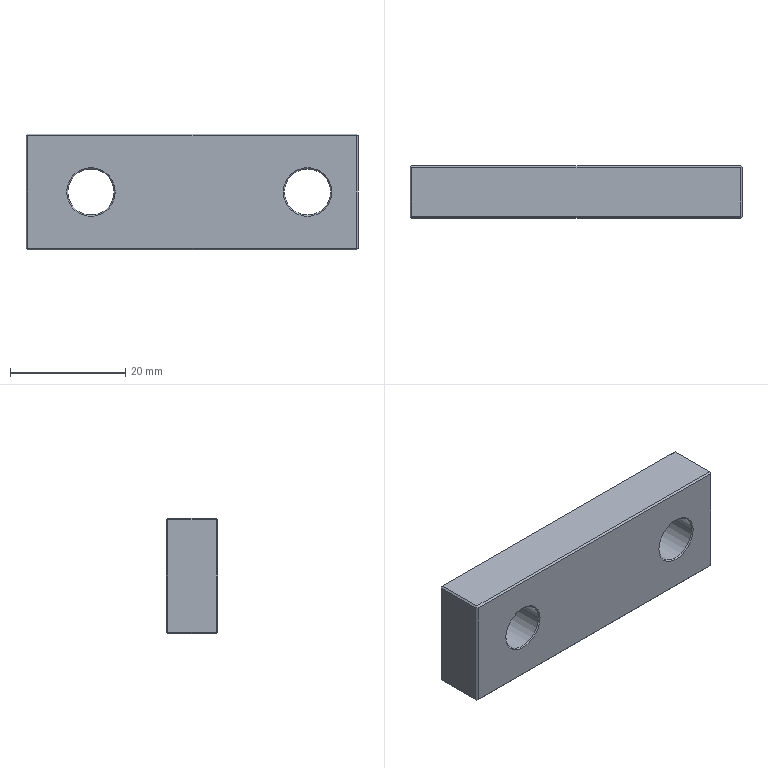Part | 1 solid | 26 faces | box 57.5 x 9 x 20 mm | volume 9429 mm3 | plane 18 | cylinder 4 | cone 4 | commonest cylinder face diameters 8 x4
STEP:
#1=CARTESIAN_POINT('',(2209.7,120.2,40.));
#2=VERTEX_POINT('',#1);
#3=CARTESIAN_POINT('',(2209.7,111.8,40.));
#4=VERTEX_POINT('',#3);
#5=CARTESIAN_POINT('',(2209.7,116.,40.));
#6=DIRECTION('',(0.,-1.,0.));
#7=VECTOR('',#6,1000.);
#8=LINE('',#5,#7);
#9=EDGE_CURVE('',#2,#4,#8,.T.);
#10=ORIENTED_EDGE('',*,*,#9,.T.);
#11=CARTESIAN_POINT('',(2152.8,111.8,40.));
#12=VERTEX_POINT('',#11);
#13=CARTESIAN_POINT('',(2184.262,111.8,40.));
#14=DIRECTION('',(1.,0.,0.));
#15=VECTOR('',#14,1000.);
#16=LINE('',#13,#15);
#17=EDGE_CURVE('',#12,#4,#16,.T.);
#18=ORIENTED_EDGE('',*,*,#17,.F.);
#19=CARTESIAN_POINT('',(2152.8,120.2,40.));
#20=VERTEX_POINT('',#19);
#21=CARTESIAN_POINT('',(2152.8,110.5,40.));
#22=DIRECTION('',(0.,-1.,0.));
#23=VECTOR('',#22,1000.);
#24=LINE('',#21,#23);
#25=EDGE_CURVE('',#20,#12,#24,.T.);
#26=ORIENTED_EDGE('',*,*,#25,.F.);
#27=CARTESIAN_POINT('',(2184.262,120.2,40.));
#28=DIRECTION('',(-1.,0.,0.));
#29=VECTOR('',#28,1000.);
#30=LINE('',#27,#29);
#31=EDGE_CURVE('',#2,#20,#30,.T.);
#32=ORIENTED_EDGE('',*,*,#31,.F.);
#33=EDGE_LOOP('',(#10,#18,#26,#32));
#34=FACE_BOUND('',#33,.T.);
#35=CARTESIAN_POINT('',(2131.5,110.5,40.));
#36=DIRECTION('',(0.,0.,-1.));
#37=DIRECTION('',(0.,-1.,0.));
#38=AXIS2_PLACEMENT_3D('',#35,#36,#37);
#39=PLANE('',#38);
#40=ADVANCED_FACE('',(#34),#39,.T.);
#41=CARTESIAN_POINT('',(2152.5,111.8,59.7));
#42=VERTEX_POINT('',#41);
#43=CARTESIAN_POINT('',(2152.5,120.2,59.7));
#44=VERTEX_POINT('',#43);
#45=CARTESIAN_POINT('',(2152.5,110.5,59.7));
#46=DIRECTION('',(0.,1.,0.));
#47=VECTOR('',#46,1000.);
#48=LINE('',#45,#47);
#49=EDGE_CURVE('',#42,#44,#48,.T.);
#50=ORIENTED_EDGE('',*,*,#49,.T.);
#51=CARTESIAN_POINT('',(2152.5,120.2,40.3));
#52=VERTEX_POINT('',#51);
#53=CARTESIAN_POINT('',(2152.5,120.2,50.));
#54=DIRECTION('',(0.,0.,1.));
#55=VECTOR('',#54,1000.);
#56=LINE('',#53,#55);
#57=EDGE_CURVE('',#52,#44,#56,.T.);
#58=ORIENTED_EDGE('',*,*,#57,.F.);
#59=CARTESIAN_POINT('',(2152.5,111.8,40.3));
#60=VERTEX_POINT('',#59);
#61=CARTESIAN_POINT('',(2152.5,110.5,40.3));
#62=DIRECTION('',(0.,-1.,0.));
#63=VECTOR('',#62,1000.);
#64=LINE('',#61,#63);
#65=EDGE_CURVE('',#52,#60,#64,.T.);
#66=ORIENTED_EDGE('',*,*,#65,.T.);
#67=CARTESIAN_POINT('',(2152.5,111.8,50.));
#68=DIRECTION('',(0.,0.,-1.));
#69=VECTOR('',#68,1000.);
#70=LINE('',#67,#69);
#71=EDGE_CURVE('',#42,#60,#70,.T.);
#72=ORIENTED_EDGE('',*,*,#71,.F.);
#73=EDGE_LOOP('',(#50,#58,#66,#72));
#74=FACE_BOUND('',#73,.T.);
#75=CARTESIAN_POINT('',(2152.5,110.5,62.5));
#76=DIRECTION('',(-1.,0.,0.));
#77=DIRECTION('',(0.,0.,1.));
#78=AXIS2_PLACEMENT_3D('',#75,#76,#77);
#79=PLANE('',#78);
#80=ADVANCED_FACE('',(#74),#79,.T.);
#81=CARTESIAN_POINT('',(2209.7,111.8,60.));
#82=VERTEX_POINT('',#81);
#83=CARTESIAN_POINT('',(2209.7,120.2,60.));
#84=VERTEX_POINT('',#83);
#85=CARTESIAN_POINT('',(2209.7,116.,60.));
#86=DIRECTION('',(0.,1.,0.));
#87=VECTOR('',#86,1000.);
#88=LINE('',#85,#87);
#89=EDGE_CURVE('',#82,#84,#88,.T.);
#90=ORIENTED_EDGE('',*,*,#89,.T.);
#91=CARTESIAN_POINT('',(2152.8,120.2,60.));
#92=VERTEX_POINT('',#91);
#93=CARTESIAN_POINT('',(2184.262,120.2,60.));
#94=DIRECTION('',(1.,0.,0.));
#95=VECTOR('',#94,1000.);
#96=LINE('',#93,#95);
#97=EDGE_CURVE('',#92,#84,#96,.T.);
#98=ORIENTED_EDGE('',*,*,#97,.F.);
#99=CARTESIAN_POINT('',(2152.8,111.8,60.));
#100=VERTEX_POINT('',#99);
#101=CARTESIAN_POINT('',(2152.8,110.5,60.));
#102=DIRECTION('',(0.,1.,0.));
#103=VECTOR('',#102,1000.);
#104=LINE('',#101,#103);
#105=EDGE_CURVE('',#100,#92,#104,.T.);
#106=ORIENTED_EDGE('',*,*,#105,.F.);
#107=CARTESIAN_POINT('',(2184.262,111.8,60.));
#108=DIRECTION('',(-1.,0.,0.));
#109=VECTOR('',#108,1000.);
#110=LINE('',#107,#109);
#111=EDGE_CURVE('',#82,#100,#110,.T.);
#112=ORIENTED_EDGE('',*,*,#111,.F.);
#113=EDGE_LOOP('',(#90,#98,#106,#112));
#114=FACE_BOUND('',#113,.T.);
#115=CARTESIAN_POINT('',(2233.5,110.5,60.));
#116=DIRECTION('',(0.,0.,1.));
#117=DIRECTION('',(1.,0.,0.));
#118=AXIS2_PLACEMENT_3D('',#115,#116,#117);
#119=PLANE('',#118);
#120=ADVANCED_FACE('',(#114),#119,.T.);
#121=CARTESIAN_POINT('',(2210.,111.8,59.7));
#122=VERTEX_POINT('',#121);
#123=CARTESIAN_POINT('',(2210.,120.2,59.7));
#124=VERTEX_POINT('',#123);
#125=CARTESIAN_POINT('',(2210.,116.,59.7));
#126=DIRECTION('',(0.,1.,0.));
#127=VECTOR('',#126,1000.);
#128=LINE('',#125,#127);
#129=EDGE_CURVE('',#122,#124,#128,.T.);
#130=ORIENTED_EDGE('',*,*,#129,.F.);
#131=CARTESIAN_POINT('',(2210.,111.8,40.3));
#132=VERTEX_POINT('',#131);
#133=CARTESIAN_POINT('',(2210.,111.8,50.));
#134=DIRECTION('',(0.,0.,-1.));
#135=VECTOR('',#134,1000.);
#136=LINE('',#133,#135);
#137=EDGE_CURVE('',#122,#132,#136,.T.);
#138=ORIENTED_EDGE('',*,*,#137,.T.);
#139=CARTESIAN_POINT('',(2210.,120.2,40.3));
#140=VERTEX_POINT('',#139);
#141=CARTESIAN_POINT('',(2210.,116.,40.3));
#142=DIRECTION('',(0.,-1.,0.));
#143=VECTOR('',#142,1000.);
#144=LINE('',#141,#143);
#145=EDGE_CURVE('',#140,#132,#144,.T.);
#146=ORIENTED_EDGE('',*,*,#145,.F.);
#147=CARTESIAN_POINT('',(2210.,120.2,50.));
#148=DIRECTION('',(0.,0.,-1.));
#149=VECTOR('',#148,1000.);
#150=LINE('',#147,#149);
#151=EDGE_CURVE('',#124,#140,#150,.T.);
#152=ORIENTED_EDGE('',*,*,#151,.F.);
#153=EDGE_LOOP('',(#130,#138,#146,#152));
#154=FACE_BOUND('',#153,.T.);
#155=CARTESIAN_POINT('',(2210.,110.5,-72.5));
#156=DIRECTION('',(1.,0.,0.));
#157=DIRECTION('',(0.,1.,0.));
#158=AXIS2_PLACEMENT_3D('',#155,#156,#157);
#159=PLANE('',#158);
#160=ADVANCED_FACE('',(#154),#159,.T.);
#161=CARTESIAN_POINT('',(2197.25,111.7,50.));
#162=VERTEX_POINT('',#161);
#163=CARTESIAN_POINT('',(2205.25,111.7,50.));
#164=VERTEX_POINT('',#163);
#165=CARTESIAN_POINT('',(2201.25,111.7,50.));
#166=DIRECTION('',(0.,-1.,0.));
#167=DIRECTION('',(1.,0.,0.));
#168=AXIS2_PLACEMENT_3D('',#165,#166,#167);
#169=CIRCLE('',#168,4.);
#170=EDGE_CURVE('',#162,#164,#169,.T.);
#171=ORIENTED_EDGE('',*,*,#170,.T.);
#172=CARTESIAN_POINT('',(2205.25,120.5,50.));
#173=VERTEX_POINT('',#172);
#174=CARTESIAN_POINT('',(2205.25,105.5,50.));
#175=DIRECTION('',(0.,-1.,0.));
#176=VECTOR('',#175,1000.);
#177=LINE('',#174,#176);
#178=EDGE_CURVE('',#173,#164,#177,.T.);
#179=ORIENTED_EDGE('',*,*,#178,.F.);
#180=CARTESIAN_POINT('',(2197.25,120.5,50.));
#181=VERTEX_POINT('',#180);
#182=CARTESIAN_POINT('',(2201.25,120.5,50.));
#183=DIRECTION('',(0.,-1.,0.));
#184=DIRECTION('',(1.,0.,0.));
#185=AXIS2_PLACEMENT_3D('',#182,#183,#184);
#186=CIRCLE('',#185,4.);
#187=EDGE_CURVE('',#181,#173,#186,.T.);
#188=ORIENTED_EDGE('',*,*,#187,.F.);
#189=CARTESIAN_POINT('',(2197.25,105.5,50.));
#190=DIRECTION('',(0.,-1.,0.));
#191=VECTOR('',#190,1000.);
#192=LINE('',#189,#191);
#193=EDGE_CURVE('',#181,#162,#192,.T.);
#194=ORIENTED_EDGE('',*,*,#193,.T.);
#195=EDGE_LOOP('',(#171,#179,#188,#194));
#196=FACE_BOUND('',#195,.T.);
#197=CARTESIAN_POINT('',(2201.25,105.5,50.));
#198=DIRECTION('',(0.,-1.,0.));
#199=DIRECTION('',(1.,0.,0.));
#200=AXIS2_PLACEMENT_3D('',#197,#198,#199);
#201=CYLINDRICAL_SURFACE('',#200,4.);
#202=ADVANCED_FACE('',(#196),#201,.F.);
#203=ORIENTED_EDGE('',*,*,#89,.F.);
#204=CARTESIAN_POINT('',(2209.85,111.65,59.85));
#205=VERTEX_POINT('',#204);
#206=CARTESIAN_POINT('',(2211.,110.5,58.7));
#207=DIRECTION('',(0.5774,-0.5774,-0.5774));
#208=VECTOR('',#207,1000.);
#209=LINE('',#206,#208);
#210=EDGE_CURVE('',#82,#205,#209,.T.);
#211=ORIENTED_EDGE('',*,*,#210,.T.);
#212=CARTESIAN_POINT('',(2302.588,204.388,-32.888));
#213=DIRECTION('',(-0.5774,-0.5774,0.5774));
#214=VECTOR('',#213,1000.);
#215=LINE('',#212,#214);
#216=EDGE_CURVE('',#122,#205,#215,.T.);
#217=ORIENTED_EDGE('',*,*,#216,.F.);
#218=ORIENTED_EDGE('',*,*,#129,.T.);
#219=CARTESIAN_POINT('',(2209.85,120.35,59.85));
#220=VERTEX_POINT('',#219);
#221=CARTESIAN_POINT('',(2302.588,27.612,-32.888));
#222=DIRECTION('',(0.5774,-0.5774,-0.5774));
#223=VECTOR('',#222,1000.);
#224=LINE('',#221,#223);
#225=EDGE_CURVE('',#220,#124,#224,.T.);
#226=ORIENTED_EDGE('',*,*,#225,.F.);
#227=CARTESIAN_POINT('',(2200.,110.5,69.7));
#228=DIRECTION('',(-0.5774,-0.5774,0.5774));
#229=VECTOR('',#228,1000.);
#230=LINE('',#227,#229);
#231=EDGE_CURVE('',#220,#84,#230,.T.);
#232=ORIENTED_EDGE('',*,*,#231,.T.);
#233=EDGE_LOOP('',(#203,#211,#217,#218,#226,#232));
#234=FACE_BOUND('',#233,.T.);
#235=CARTESIAN_POINT('',(2209.85,116.,59.85));
#236=DIRECTION('',(0.7071,0.,0.7071));
#237=DIRECTION('',(0.,-1.,0.));
#238=AXIS2_PLACEMENT_3D('',#235,#236,#237);
#239=PLANE('',#238);
#240=ADVANCED_FACE('',(#234),#239,.T.);
#241=ORIENTED_EDGE('',*,*,#25,.T.);
#242=CARTESIAN_POINT('',(2152.65,111.65,40.15));
#243=VERTEX_POINT('',#242);
#244=CARTESIAN_POINT('',(2184.262,143.262,8.538));
#245=DIRECTION('',(-0.5774,-0.5774,0.5774));
#246=VECTOR('',#245,1000.);
#247=LINE('',#244,#246);
#248=EDGE_CURVE('',#12,#243,#247,.T.);
#249=ORIENTED_EDGE('',*,*,#248,.T.);
#250=CARTESIAN_POINT('',(2184.262,80.038,8.538));
#251=DIRECTION('',(-0.5774,0.5774,0.5774));
#252=VECTOR('',#251,1000.);
#253=LINE('',#250,#252);
#254=EDGE_CURVE('',#243,#60,#253,.T.);
#255=ORIENTED_EDGE('',*,*,#254,.T.);
#256=ORIENTED_EDGE('',*,*,#65,.F.);
#257=CARTESIAN_POINT('',(2152.65,120.35,40.15));
#258=VERTEX_POINT('',#257);
#259=CARTESIAN_POINT('',(2184.262,151.962,8.538));
#260=DIRECTION('',(-0.5774,-0.5774,0.5774));
#261=VECTOR('',#260,1000.);
#262=LINE('',#259,#261);
#263=EDGE_CURVE('',#258,#52,#262,.T.);
#264=ORIENTED_EDGE('',*,*,#263,.F.);
#265=CARTESIAN_POINT('',(2162.5,110.5,30.3));
#266=DIRECTION('',(-0.5774,0.5774,0.5774));
#267=VECTOR('',#266,1000.);
#268=LINE('',#265,#267);
#269=EDGE_CURVE('',#20,#258,#268,.T.);
#270=ORIENTED_EDGE('',*,*,#269,.F.);
#271=EDGE_LOOP('',(#241,#249,#255,#256,#264,#270));
#272=FACE_BOUND('',#271,.T.);
#273=CARTESIAN_POINT('',(2152.65,114.5,40.15));
#274=DIRECTION('',(0.7071,0.,0.7071));
#275=DIRECTION('',(0.,-1.,0.));
#276=AXIS2_PLACEMENT_3D('',#273,#274,#275);
#277=PLANE('',#276);
#278=ADVANCED_FACE('',(#272),#277,.F.);
#279=ORIENTED_EDGE('',*,*,#49,.F.);
#280=CARTESIAN_POINT('',(2152.65,111.65,59.85));
#281=VERTEX_POINT('',#280);
#282=CARTESIAN_POINT('',(2184.262,80.038,91.462));
#283=DIRECTION('',(-0.5774,0.5774,-0.5774));
#284=VECTOR('',#283,1000.);
#285=LINE('',#282,#284);
#286=EDGE_CURVE('',#281,#42,#285,.T.);
#287=ORIENTED_EDGE('',*,*,#286,.F.);
#288=CARTESIAN_POINT('',(2151.5,110.5,58.7));
#289=DIRECTION('',(-0.5774,-0.5774,-0.5774));
#290=VECTOR('',#289,1000.);
#291=LINE('',#288,#290);
#292=EDGE_CURVE('',#100,#281,#291,.T.);
#293=ORIENTED_EDGE('',*,*,#292,.F.);
#294=ORIENTED_EDGE('',*,*,#105,.T.);
#295=CARTESIAN_POINT('',(2152.65,120.35,59.85));
#296=VERTEX_POINT('',#295);
#297=CARTESIAN_POINT('',(2162.5,110.5,69.7));
#298=DIRECTION('',(-0.5774,0.5774,-0.5774));
#299=VECTOR('',#298,1000.);
#300=LINE('',#297,#299);
#301=EDGE_CURVE('',#92,#296,#300,.T.);
#302=ORIENTED_EDGE('',*,*,#301,.T.);
#303=CARTESIAN_POINT('',(2142.8,110.5,50.));
#304=DIRECTION('',(0.5774,0.5774,0.5774));
#305=VECTOR('',#304,1000.);
#306=LINE('',#303,#305);
#307=EDGE_CURVE('',#44,#296,#306,.T.);
#308=ORIENTED_EDGE('',*,*,#307,.F.);
#309=EDGE_LOOP('',(#279,#287,#293,#294,#302,#308));
#310=FACE_BOUND('',#309,.T.);
#311=CARTESIAN_POINT('',(2152.65,114.5,59.85));
#312=DIRECTION('',(-0.7071,0.,0.7071));
#313=DIRECTION('',(0.,1.,0.));
#314=AXIS2_PLACEMENT_3D('',#311,#312,#313);
#315=PLANE('',#314);
#316=ADVANCED_FACE('',(#310),#315,.T.);
#317=ORIENTED_EDGE('',*,*,#9,.F.);
#318=CARTESIAN_POINT('',(2209.85,120.35,40.15));
#319=VERTEX_POINT('',#318);
#320=CARTESIAN_POINT('',(2200.,110.5,30.3));
#321=DIRECTION('',(0.5774,0.5774,0.5774));
#322=VECTOR('',#321,1000.);
#323=LINE('',#320,#322);
#324=EDGE_CURVE('',#2,#319,#323,.T.);
#325=ORIENTED_EDGE('',*,*,#324,.T.);
#326=CARTESIAN_POINT('',(2219.7,110.5,50.));
#327=DIRECTION('',(-0.5774,0.5774,-0.5774));
#328=VECTOR('',#327,1000.);
#329=LINE('',#326,#328);
#330=EDGE_CURVE('',#140,#319,#329,.T.);
#331=ORIENTED_EDGE('',*,*,#330,.F.);
#332=ORIENTED_EDGE('',*,*,#145,.T.);
#333=CARTESIAN_POINT('',(2209.85,111.65,40.15));
#334=VERTEX_POINT('',#333);
#335=CARTESIAN_POINT('',(2184.262,86.062,14.562));
#336=DIRECTION('',(-0.5774,-0.5774,-0.5774));
#337=VECTOR('',#336,1000.);
#338=LINE('',#335,#337);
#339=EDGE_CURVE('',#132,#334,#338,.T.);
#340=ORIENTED_EDGE('',*,*,#339,.T.);
#341=CARTESIAN_POINT('',(2211.,110.5,41.3));
#342=DIRECTION('',(-0.5774,0.5774,-0.5774));
#343=VECTOR('',#342,1000.);
#344=LINE('',#341,#343);
#345=EDGE_CURVE('',#334,#4,#344,.T.);
#346=ORIENTED_EDGE('',*,*,#345,.T.);
#347=EDGE_LOOP('',(#317,#325,#331,#332,#340,#346));
#348=FACE_BOUND('',#347,.T.);
#349=CARTESIAN_POINT('',(2209.85,116.,40.15));
#350=DIRECTION('',(0.7071,0.,-0.7071));
#351=DIRECTION('',(0.,-1.,0.));
#352=AXIS2_PLACEMENT_3D('',#349,#350,#351);
#353=PLANE('',#352);
#354=ADVANCED_FACE('',(#348),#353,.T.);
#355=ORIENTED_EDGE('',*,*,#170,.F.);
#356=CARTESIAN_POINT('',(2197.05,111.5,50.));
#357=VERTEX_POINT('',#356);
#358=CARTESIAN_POINT('',(2197.25,111.7,50.));
#359=DIRECTION('',(-0.7071,-0.7071,0.));
#360=VECTOR('',#359,1000.);
#361=LINE('',#358,#360);
#362=EDGE_CURVE('',#162,#357,#361,.T.);
#363=ORIENTED_EDGE('',*,*,#362,.T.);
#364=CARTESIAN_POINT('',(2205.45,111.5,50.));
#365=VERTEX_POINT('',#364);
#366=CARTESIAN_POINT('',(2201.25,111.5,50.));
#367=DIRECTION('',(0.,-1.,0.));
#368=DIRECTION('',(1.,0.,0.));
#369=AXIS2_PLACEMENT_3D('',#366,#367,#368);
#370=CIRCLE('',#369,4.2);
#371=EDGE_CURVE('',#357,#365,#370,.T.);
#372=ORIENTED_EDGE('',*,*,#371,.T.);
#373=CARTESIAN_POINT('',(2205.25,111.7,50.));
#374=DIRECTION('',(0.7071,-0.7071,0.));
#375=VECTOR('',#374,1000.);
#376=LINE('',#373,#375);
#377=EDGE_CURVE('',#164,#365,#376,.T.);
#378=ORIENTED_EDGE('',*,*,#377,.F.);
#379=EDGE_LOOP('',(#355,#363,#372,#378));
#380=FACE_BOUND('',#379,.T.);
#381=CARTESIAN_POINT('',(2201.25,111.7,50.));
#382=DIRECTION('',(0.,-1.,0.));
#383=DIRECTION('',(1.,0.,0.));
#384=AXIS2_PLACEMENT_3D('',#381,#382,#383);
#385=CONICAL_SURFACE('',#384,4.,0.7854);
#386=ADVANCED_FACE('',(#380),#385,.F.);
#387=ORIENTED_EDGE('',*,*,#178,.T.);
#388=CARTESIAN_POINT('',(2201.25,111.7,50.));
#389=DIRECTION('',(0.,-1.,0.));
#390=DIRECTION('',(1.,0.,0.));
#391=AXIS2_PLACEMENT_3D('',#388,#389,#390);
#392=CIRCLE('',#391,4.);
#393=EDGE_CURVE('',#164,#162,#392,.T.);
#394=ORIENTED_EDGE('',*,*,#393,.T.);
#395=ORIENTED_EDGE('',*,*,#193,.F.);
#396=CARTESIAN_POINT('',(2201.25,120.5,50.));
#397=DIRECTION('',(0.,-1.,0.));
#398=DIRECTION('',(1.,0.,0.));
#399=AXIS2_PLACEMENT_3D('',#396,#397,#398);
#400=CIRCLE('',#399,4.);
#401=EDGE_CURVE('',#173,#181,#400,.T.);
#402=ORIENTED_EDGE('',*,*,#401,.F.);
#403=EDGE_LOOP('',(#387,#394,#395,#402));
#404=FACE_BOUND('',#403,.T.);
#405=CARTESIAN_POINT('',(2201.25,105.5,50.));
#406=DIRECTION('',(0.,-1.,0.));
#407=DIRECTION('',(1.,0.,0.));
#408=AXIS2_PLACEMENT_3D('',#405,#406,#407);
#409=CYLINDRICAL_SURFACE('',#408,4.);
#410=ADVANCED_FACE('',(#404),#409,.F.);
#411=ORIENTED_EDGE('',*,*,#377,.T.);
#412=CARTESIAN_POINT('',(2201.25,111.5,50.));
#413=DIRECTION('',(0.,-1.,0.));
#414=DIRECTION('',(1.,0.,0.));
#415=AXIS2_PLACEMENT_3D('',#412,#413,#414);
#416=CIRCLE('',#415,4.2);
#417=EDGE_CURVE('',#365,#357,#416,.T.);
#418=ORIENTED_EDGE('',*,*,#417,.T.);
#419=ORIENTED_EDGE('',*,*,#362,.F.);
#420=ORIENTED_EDGE('',*,*,#393,.F.);
#421=EDGE_LOOP('',(#411,#418,#419,#420));
#422=FACE_BOUND('',#421,.T.);
#423=CARTESIAN_POINT('',(2201.25,111.7,50.));
#424=DIRECTION('',(0.,-1.,0.));
#425=DIRECTION('',(1.,0.,0.));
#426=AXIS2_PLACEMENT_3D('',#423,#424,#425);
#427=CONICAL_SURFACE('',#426,4.,0.7854);
#428=ADVANCED_FACE('',(#422),#427,.F.);
#429=CARTESIAN_POINT('',(2209.7,120.5,59.7));
#430=VERTEX_POINT('',#429);
#431=CARTESIAN_POINT('',(2209.7,120.5,40.3));
#432=VERTEX_POINT('',#431);
#433=CARTESIAN_POINT('',(2209.7,120.5,50.));
#434=DIRECTION('',(0.,0.,-1.));
#435=VECTOR('',#434,1000.);
#436=LINE('',#433,#435);
#437=EDGE_CURVE('',#430,#432,#436,.T.);
#438=ORIENTED_EDGE('',*,*,#437,.T.);
#439=CARTESIAN_POINT('',(2152.8,120.5,40.3));
#440=VERTEX_POINT('',#439);
#441=CARTESIAN_POINT('',(2184.262,120.5,40.3));
#442=DIRECTION('',(-1.,0.,0.));
#443=VECTOR('',#442,1000.);
#444=LINE('',#441,#443);
#445=EDGE_CURVE('',#432,#440,#444,.T.);
#446=ORIENTED_EDGE('',*,*,#445,.T.);
#447=CARTESIAN_POINT('',(2152.8,120.5,59.7));
#448=VERTEX_POINT('',#447);
#449=CARTESIAN_POINT('',(2152.8,120.5,50.));
#450=DIRECTION('',(0.,0.,1.));
#451=VECTOR('',#450,1000.);
#452=LINE('',#449,#451);
#453=EDGE_CURVE('',#440,#448,#452,.T.);
#454=ORIENTED_EDGE('',*,*,#453,.T.);
#455=CARTESIAN_POINT('',(2184.262,120.5,59.7));
#456=DIRECTION('',(1.,0.,0.));
#457=VECTOR('',#456,1000.);
#458=LINE('',#455,#457);
#459=EDGE_CURVE('',#448,#430,#458,.T.);
#460=ORIENTED_EDGE('',*,*,#459,.T.);
#461=EDGE_LOOP('',(#438,#446,#454,#460));
#462=FACE_BOUND('',#461,.T.);
#463=ORIENTED_EDGE('',*,*,#187,.T.);
#464=ORIENTED_EDGE('',*,*,#401,.T.);
#465=EDGE_LOOP('',(#463,#464));
#466=FACE_BOUND('',#465,.T.);
#467=CARTESIAN_POINT('',(2159.75,120.5,50.));
#468=VERTEX_POINT('',#467);
#469=CARTESIAN_POINT('',(2167.75,120.5,50.));
#470=VERTEX_POINT('',#469);
#471=CARTESIAN_POINT('',(2163.75,120.5,50.));
#472=DIRECTION('',(0.,-1.,0.));
#473=DIRECTION('',(1.,0.,0.));
#474=AXIS2_PLACEMENT_3D('',#471,#472,#473);
#475=CIRCLE('',#474,4.);
#476=EDGE_CURVE('',#468,#470,#475,.T.);
#477=ORIENTED_EDGE('',*,*,#476,.T.);
#478=CARTESIAN_POINT('',(2163.75,120.5,50.));
#479=DIRECTION('',(0.,-1.,0.));
#480=DIRECTION('',(1.,0.,0.));
#481=AXIS2_PLACEMENT_3D('',#478,#479,#480);
#482=CIRCLE('',#481,4.);
#483=EDGE_CURVE('',#470,#468,#482,.T.);
#484=ORIENTED_EDGE('',*,*,#483,.T.);
#485=EDGE_LOOP('',(#477,#484));
#486=FACE_BOUND('',#485,.T.);
#487=CARTESIAN_POINT('',(2184.262,120.5,-32.888));
#488=DIRECTION('',(0.,1.,0.));
#489=DIRECTION('',(1.,0.,0.));
#490=AXIS2_PLACEMENT_3D('',#487,#488,#489);
#491=PLANE('',#490);
#492=ADVANCED_FACE('',(#462,#466,#486),#491,.T.);
#493=CARTESIAN_POINT('',(2159.75,111.7,50.));
#494=VERTEX_POINT('',#493);
#495=CARTESIAN_POINT('',(2167.75,111.7,50.));
#496=VERTEX_POINT('',#495);
#497=CARTESIAN_POINT('',(2163.75,111.7,50.));
#498=DIRECTION('',(0.,-1.,0.));
#499=DIRECTION('',(1.,0.,0.));
#500=AXIS2_PLACEMENT_3D('',#497,#498,#499);
#501=CIRCLE('',#500,4.);
#502=EDGE_CURVE('',#494,#496,#501,.T.);
#503=ORIENTED_EDGE('',*,*,#502,.T.);
#504=CARTESIAN_POINT('',(2167.75,105.5,50.));
#505=DIRECTION('',(0.,-1.,0.));
#506=VECTOR('',#505,1000.);
#507=LINE('',#504,#506);
#508=EDGE_CURVE('',#470,#496,#507,.T.);
#509=ORIENTED_EDGE('',*,*,#508,.F.);
#510=ORIENTED_EDGE('',*,*,#476,.F.);
#511=CARTESIAN_POINT('',(2159.75,105.5,50.));
#512=DIRECTION('',(0.,-1.,0.));
#513=VECTOR('',#512,1000.);
#514=LINE('',#511,#513);
#515=EDGE_CURVE('',#468,#494,#514,.T.);
#516=ORIENTED_EDGE('',*,*,#515,.T.);
#517=EDGE_LOOP('',(#503,#509,#510,#516));
#518=FACE_BOUND('',#517,.T.);
#519=CARTESIAN_POINT('',(2163.75,105.5,50.));
#520=DIRECTION('',(0.,-1.,0.));
#521=DIRECTION('',(1.,0.,0.));
#522=AXIS2_PLACEMENT_3D('',#519,#520,#521);
#523=CYLINDRICAL_SURFACE('',#522,4.);
#524=ADVANCED_FACE('',(#518),#523,.F.);
#525=ORIENTED_EDGE('',*,*,#437,.F.);
#526=CARTESIAN_POINT('',(2219.7,110.5,69.7));
#527=DIRECTION('',(0.5774,-0.5774,0.5774));
#528=VECTOR('',#527,1000.);
#529=LINE('',#526,#528);
#530=EDGE_CURVE('',#430,#220,#529,.T.);
#531=ORIENTED_EDGE('',*,*,#530,.T.);
#532=ORIENTED_EDGE('',*,*,#225,.T.);
#533=ORIENTED_EDGE('',*,*,#151,.T.);
#534=ORIENTED_EDGE('',*,*,#330,.T.);
#535=CARTESIAN_POINT('',(2219.7,110.5,30.3));
#536=DIRECTION('',(-0.5774,0.5774,0.5774));
#537=VECTOR('',#536,1000.);
#538=LINE('',#535,#537);
#539=EDGE_CURVE('',#319,#432,#538,.T.);
#540=ORIENTED_EDGE('',*,*,#539,.T.);
#541=EDGE_LOOP('',(#525,#531,#532,#533,#534,#540));
#542=FACE_BOUND('',#541,.T.);
#543=CARTESIAN_POINT('',(2209.85,120.35,50.));
#544=DIRECTION('',(0.7071,0.7071,0.));
#545=DIRECTION('',(0.,0.,-1.));
#546=AXIS2_PLACEMENT_3D('',#543,#544,#545);
#547=PLANE('',#546);
#548=ADVANCED_FACE('',(#542),#547,.T.);
#549=ORIENTED_EDGE('',*,*,#445,.F.);
#550=ORIENTED_EDGE('',*,*,#539,.F.);
#551=ORIENTED_EDGE('',*,*,#324,.F.);
#552=ORIENTED_EDGE('',*,*,#31,.T.);
#553=ORIENTED_EDGE('',*,*,#269,.T.);
#554=CARTESIAN_POINT('',(2142.8,110.5,30.3));
#555=DIRECTION('',(0.5774,0.5774,0.5774));
#556=VECTOR('',#555,1000.);
#557=LINE('',#554,#556);
#558=EDGE_CURVE('',#258,#440,#557,.T.);
#559=ORIENTED_EDGE('',*,*,#558,.T.);
#560=EDGE_LOOP('',(#549,#550,#551,#552,#553,#559));
#561=FACE_BOUND('',#560,.T.);
#562=CARTESIAN_POINT('',(2182.5,120.35,40.15));
#563=DIRECTION('',(0.,0.7071,-0.7071));
#564=DIRECTION('',(-1.,0.,0.));
#565=AXIS2_PLACEMENT_3D('',#562,#563,#564);
#566=PLANE('',#565);
#567=ADVANCED_FACE('',(#561),#566,.T.);
#568=ORIENTED_EDGE('',*,*,#453,.F.);
#569=ORIENTED_EDGE('',*,*,#558,.F.);
#570=ORIENTED_EDGE('',*,*,#263,.T.);
#571=ORIENTED_EDGE('',*,*,#57,.T.);
#572=ORIENTED_EDGE('',*,*,#307,.T.);
#573=CARTESIAN_POINT('',(2142.8,110.5,69.7));
#574=DIRECTION('',(0.5774,0.5774,-0.5774));
#575=VECTOR('',#574,1000.);
#576=LINE('',#573,#575);
#577=EDGE_CURVE('',#296,#448,#576,.T.);
#578=ORIENTED_EDGE('',*,*,#577,.T.);
#579=EDGE_LOOP('',(#568,#569,#570,#571,#572,#578));
#580=FACE_BOUND('',#579,.T.);
#581=CARTESIAN_POINT('',(2152.65,120.35,50.));
#582=DIRECTION('',(-0.7071,0.7071,0.));
#583=DIRECTION('',(0.,0.,1.));
#584=AXIS2_PLACEMENT_3D('',#581,#582,#583);
#585=PLANE('',#584);
#586=ADVANCED_FACE('',(#580),#585,.T.);
#587=ORIENTED_EDGE('',*,*,#97,.T.);
#588=ORIENTED_EDGE('',*,*,#231,.F.);
#589=ORIENTED_EDGE('',*,*,#530,.F.);
#590=ORIENTED_EDGE('',*,*,#459,.F.);
#591=ORIENTED_EDGE('',*,*,#577,.F.);
#592=ORIENTED_EDGE('',*,*,#301,.F.);
#593=EDGE_LOOP('',(#587,#588,#589,#590,#591,#592));
#594=FACE_BOUND('',#593,.T.);
#595=CARTESIAN_POINT('',(2182.5,120.35,59.85));
#596=DIRECTION('',(0.,0.7071,0.7071));
#597=DIRECTION('',(1.,0.,0.));
#598=AXIS2_PLACEMENT_3D('',#595,#596,#597);
#599=PLANE('',#598);
#600=ADVANCED_FACE('',(#594),#599,.T.);
#601=ORIENTED_EDGE('',*,*,#502,.F.);
#602=CARTESIAN_POINT('',(2159.55,111.5,50.));
#603=VERTEX_POINT('',#602);
#604=CARTESIAN_POINT('',(2159.75,111.7,50.));
#605=DIRECTION('',(-0.7071,-0.7071,0.));
#606=VECTOR('',#605,1000.);
#607=LINE('',#604,#606);
#608=EDGE_CURVE('',#494,#603,#607,.T.);
#609=ORIENTED_EDGE('',*,*,#608,.T.);
#610=CARTESIAN_POINT('',(2167.95,111.5,50.));
#611=VERTEX_POINT('',#610);
#612=CARTESIAN_POINT('',(2163.75,111.5,50.));
#613=DIRECTION('',(0.,-1.,0.));
#614=DIRECTION('',(1.,0.,0.));
#615=AXIS2_PLACEMENT_3D('',#612,#613,#614);
#616=CIRCLE('',#615,4.2);
#617=EDGE_CURVE('',#603,#611,#616,.T.);
#618=ORIENTED_EDGE('',*,*,#617,.T.);
#619=CARTESIAN_POINT('',(2167.75,111.7,50.));
#620=DIRECTION('',(0.7071,-0.7071,0.));
#621=VECTOR('',#620,1000.);
#622=LINE('',#619,#621);
#623=EDGE_CURVE('',#496,#611,#622,.T.);
#624=ORIENTED_EDGE('',*,*,#623,.F.);
#625=EDGE_LOOP('',(#601,#609,#618,#624));
#626=FACE_BOUND('',#625,.T.);
#627=CARTESIAN_POINT('',(2163.75,111.7,50.));
#628=DIRECTION('',(0.,-1.,0.));
#629=DIRECTION('',(1.,0.,0.));
#630=AXIS2_PLACEMENT_3D('',#627,#628,#629);
#631=CONICAL_SURFACE('',#630,4.,0.7854);
#632=ADVANCED_FACE('',(#626),#631,.F.);
#633=ORIENTED_EDGE('',*,*,#623,.T.);
#634=CARTESIAN_POINT('',(2163.75,111.5,50.));
#635=DIRECTION('',(0.,-1.,0.));
#636=DIRECTION('',(1.,0.,0.));
#637=AXIS2_PLACEMENT_3D('',#634,#635,#636);
#638=CIRCLE('',#637,4.2);
#639=EDGE_CURVE('',#611,#603,#638,.T.);
#640=ORIENTED_EDGE('',*,*,#639,.T.);
#641=ORIENTED_EDGE('',*,*,#608,.F.);
#642=CARTESIAN_POINT('',(2163.75,111.7,50.));
#643=DIRECTION('',(0.,-1.,0.));
#644=DIRECTION('',(1.,0.,0.));
#645=AXIS2_PLACEMENT_3D('',#642,#643,#644);
#646=CIRCLE('',#645,4.);
#647=EDGE_CURVE('',#496,#494,#646,.T.);
#648=ORIENTED_EDGE('',*,*,#647,.F.);
#649=EDGE_LOOP('',(#633,#640,#641,#648));
#650=FACE_BOUND('',#649,.T.);
#651=CARTESIAN_POINT('',(2163.75,111.7,50.));
#652=DIRECTION('',(0.,-1.,0.));
#653=DIRECTION('',(1.,0.,0.));
#654=AXIS2_PLACEMENT_3D('',#651,#652,#653);
#655=CONICAL_SURFACE('',#654,4.,0.7854);
#656=ADVANCED_FACE('',(#650),#655,.F.);
#657=ORIENTED_EDGE('',*,*,#508,.T.);
#658=ORIENTED_EDGE('',*,*,#647,.T.);
#659=ORIENTED_EDGE('',*,*,#515,.F.);
#660=ORIENTED_EDGE('',*,*,#483,.F.);
#661=EDGE_LOOP('',(#657,#658,#659,#660));
#662=FACE_BOUND('',#661,.T.);
#663=CARTESIAN_POINT('',(2163.75,105.5,50.));
#664=DIRECTION('',(0.,-1.,0.));
#665=DIRECTION('',(1.,0.,0.));
#666=AXIS2_PLACEMENT_3D('',#663,#664,#665);
#667=CYLINDRICAL_SURFACE('',#666,4.);
#668=ADVANCED_FACE('',(#662),#667,.F.);
#669=CARTESIAN_POINT('',(2209.7,111.5,59.7));
#670=VERTEX_POINT('',#669);
#671=CARTESIAN_POINT('',(2209.7,111.5,40.3));
#672=VERTEX_POINT('',#671);
#673=CARTESIAN_POINT('',(2209.7,111.5,50.));
#674=DIRECTION('',(0.,0.,-1.));
#675=VECTOR('',#674,1000.);
#676=LINE('',#673,#675);
#677=EDGE_CURVE('',#670,#672,#676,.T.);
#678=ORIENTED_EDGE('',*,*,#677,.F.);
#679=CARTESIAN_POINT('',(2152.8,111.5,59.7));
#680=VERTEX_POINT('',#679);
#681=CARTESIAN_POINT('',(2184.262,111.5,59.7));
#682=DIRECTION('',(-1.,0.,0.));
#683=VECTOR('',#682,1000.);
#684=LINE('',#681,#683);
#685=EDGE_CURVE('',#670,#680,#684,.T.);
#686=ORIENTED_EDGE('',*,*,#685,.T.);
#687=CARTESIAN_POINT('',(2152.8,111.5,40.3));
#688=VERTEX_POINT('',#687);
#689=CARTESIAN_POINT('',(2152.8,111.5,50.));
#690=DIRECTION('',(0.,0.,-1.));
#691=VECTOR('',#690,1000.);
#692=LINE('',#689,#691);
#693=EDGE_CURVE('',#680,#688,#692,.T.);
#694=ORIENTED_EDGE('',*,*,#693,.T.);
#695=CARTESIAN_POINT('',(2184.262,111.5,40.3));
#696=DIRECTION('',(1.,0.,0.));
#697=VECTOR('',#696,1000.);
#698=LINE('',#695,#697);
#699=EDGE_CURVE('',#688,#672,#698,.T.);
#700=ORIENTED_EDGE('',*,*,#699,.T.);
#701=EDGE_LOOP('',(#678,#686,#694,#700));
#702=FACE_BOUND('',#701,.T.);
#703=ORIENTED_EDGE('',*,*,#371,.F.);
#704=ORIENTED_EDGE('',*,*,#417,.F.);
#705=EDGE_LOOP('',(#703,#704));
#706=FACE_BOUND('',#705,.T.);
#707=ORIENTED_EDGE('',*,*,#617,.F.);
#708=ORIENTED_EDGE('',*,*,#639,.F.);
#709=EDGE_LOOP('',(#707,#708));
#710=FACE_BOUND('',#709,.T.);
#711=CARTESIAN_POINT('',(2184.262,111.5,-32.888));
#712=DIRECTION('',(0.,1.,0.));
#713=DIRECTION('',(1.,0.,0.));
#714=AXIS2_PLACEMENT_3D('',#711,#712,#713);
#715=PLANE('',#714);
#716=ADVANCED_FACE('',(#702,#706,#710),#715,.F.);
#717=ORIENTED_EDGE('',*,*,#17,.T.);
#718=ORIENTED_EDGE('',*,*,#345,.F.);
#719=CARTESIAN_POINT('',(2184.262,86.062,65.738));
#720=DIRECTION('',(-0.5774,-0.5774,0.5774));
#721=VECTOR('',#720,1000.);
#722=LINE('',#719,#721);
#723=EDGE_CURVE('',#334,#672,#722,.T.);
#724=ORIENTED_EDGE('',*,*,#723,.T.);
#725=ORIENTED_EDGE('',*,*,#699,.F.);
#726=CARTESIAN_POINT('',(2184.262,80.038,71.762));
#727=DIRECTION('',(0.5774,-0.5774,0.5774));
#728=VECTOR('',#727,1000.);
#729=LINE('',#726,#728);
#730=EDGE_CURVE('',#243,#688,#729,.T.);
#731=ORIENTED_EDGE('',*,*,#730,.F.);
#732=ORIENTED_EDGE('',*,*,#248,.F.);
#733=EDGE_LOOP('',(#717,#718,#724,#725,#731,#732));
#734=FACE_BOUND('',#733,.T.);
#735=CARTESIAN_POINT('',(2182.5,111.65,40.15));
#736=DIRECTION('',(0.,-0.7071,-0.7071));
#737=DIRECTION('',(0.,-0.7071,0.7071));
#738=AXIS2_PLACEMENT_3D('',#735,#736,#737);
#739=PLANE('',#738);
#740=ADVANCED_FACE('',(#734),#739,.T.);
#741=ORIENTED_EDGE('',*,*,#693,.F.);
#742=CARTESIAN_POINT('',(2184.262,80.038,28.238));
#743=DIRECTION('',(0.5774,-0.5774,-0.5774));
#744=VECTOR('',#743,1000.);
#745=LINE('',#742,#744);
#746=EDGE_CURVE('',#281,#680,#745,.T.);
#747=ORIENTED_EDGE('',*,*,#746,.F.);
#748=ORIENTED_EDGE('',*,*,#286,.T.);
#749=ORIENTED_EDGE('',*,*,#71,.T.);
#750=ORIENTED_EDGE('',*,*,#254,.F.);
#751=ORIENTED_EDGE('',*,*,#730,.T.);
#752=EDGE_LOOP('',(#741,#747,#748,#749,#750,#751));
#753=FACE_BOUND('',#752,.T.);
#754=CARTESIAN_POINT('',(2152.65,111.65,50.));
#755=DIRECTION('',(-0.7071,-0.7071,0.));
#756=DIRECTION('',(-0.7071,0.7071,0.));
#757=AXIS2_PLACEMENT_3D('',#754,#755,#756);
#758=PLANE('',#757);
#759=ADVANCED_FACE('',(#753),#758,.T.);
#760=ORIENTED_EDGE('',*,*,#685,.F.);
#761=CARTESIAN_POINT('',(2184.262,86.062,34.262));
#762=DIRECTION('',(0.5774,0.5774,0.5774));
#763=VECTOR('',#762,1000.);
#764=LINE('',#761,#763);
#765=EDGE_CURVE('',#670,#205,#764,.T.);
#766=ORIENTED_EDGE('',*,*,#765,.T.);
#767=ORIENTED_EDGE('',*,*,#210,.F.);
#768=ORIENTED_EDGE('',*,*,#111,.T.);
#769=ORIENTED_EDGE('',*,*,#292,.T.);
#770=ORIENTED_EDGE('',*,*,#746,.T.);
#771=EDGE_LOOP('',(#760,#766,#767,#768,#769,#770));
#772=FACE_BOUND('',#771,.T.);
#773=CARTESIAN_POINT('',(2182.5,111.65,59.85));
#774=DIRECTION('',(0.,-0.7071,0.7071));
#775=DIRECTION('',(-1.,0.,0.));
#776=AXIS2_PLACEMENT_3D('',#773,#774,#775);
#777=PLANE('',#776);
#778=ADVANCED_FACE('',(#772),#777,.T.);
#779=ORIENTED_EDGE('',*,*,#677,.T.);
#780=ORIENTED_EDGE('',*,*,#723,.F.);
#781=ORIENTED_EDGE('',*,*,#339,.F.);
#782=ORIENTED_EDGE('',*,*,#137,.F.);
#783=ORIENTED_EDGE('',*,*,#216,.T.);
#784=ORIENTED_EDGE('',*,*,#765,.F.);
#785=EDGE_LOOP('',(#779,#780,#781,#782,#783,#784));
#786=FACE_BOUND('',#785,.T.);
#787=CARTESIAN_POINT('',(2209.85,111.65,50.));
#788=DIRECTION('',(-0.7071,0.7071,0.));
#789=DIRECTION('',(0.,0.,1.));
#790=AXIS2_PLACEMENT_3D('',#787,#788,#789);
#791=PLANE('',#790);
#792=ADVANCED_FACE('',(#786),#791,.F.);
#793=CLOSED_SHELL('',(#40,#80,#120,#160,#202,#240,#278,#316,#354,#386,#410,#428,#492,#524,#548,#567,#586,#600,#632,#656,#668,#716,#740,#759,#778,#792));
#794=MANIFOLD_SOLID_BREP('',#793);
#795=(LENGTH_UNIT()NAMED_UNIT(*)SI_UNIT(.MILLI.,.METRE.));
#796=UNCERTAINTY_MEASURE_WITH_UNIT(LENGTH_MEASURE(0.00001),#795,'','');
#797=(NAMED_UNIT(*)PLANE_ANGLE_UNIT()SI_UNIT($,.RADIAN.));
#798=(NAMED_UNIT(*)SI_UNIT($,.STERADIAN.)SOLID_ANGLE_UNIT());
#799=(GEOMETRIC_REPRESENTATION_CONTEXT(3)GLOBAL_UNCERTAINTY_ASSIGNED_CONTEXT((#796))GLOBAL_UNIT_ASSIGNED_CONTEXT((#795,#797,#798))REPRESENTATION_CONTEXT('',''));
#800=ADVANCED_BREP_SHAPE_REPRESENTATION('',(#794),#799);